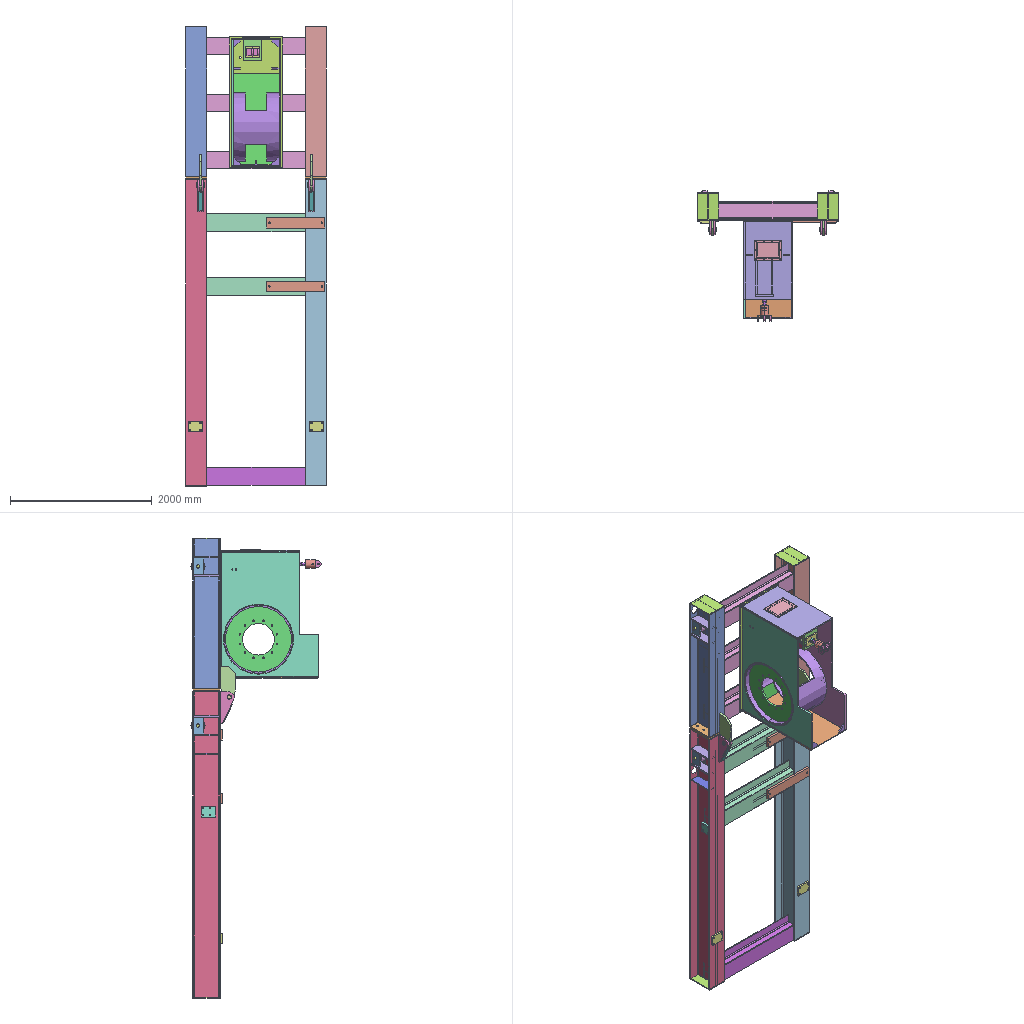Assembly | SolidWorks | 53 different items | 109 placed | box 1991 x 1839 x 6500 mm
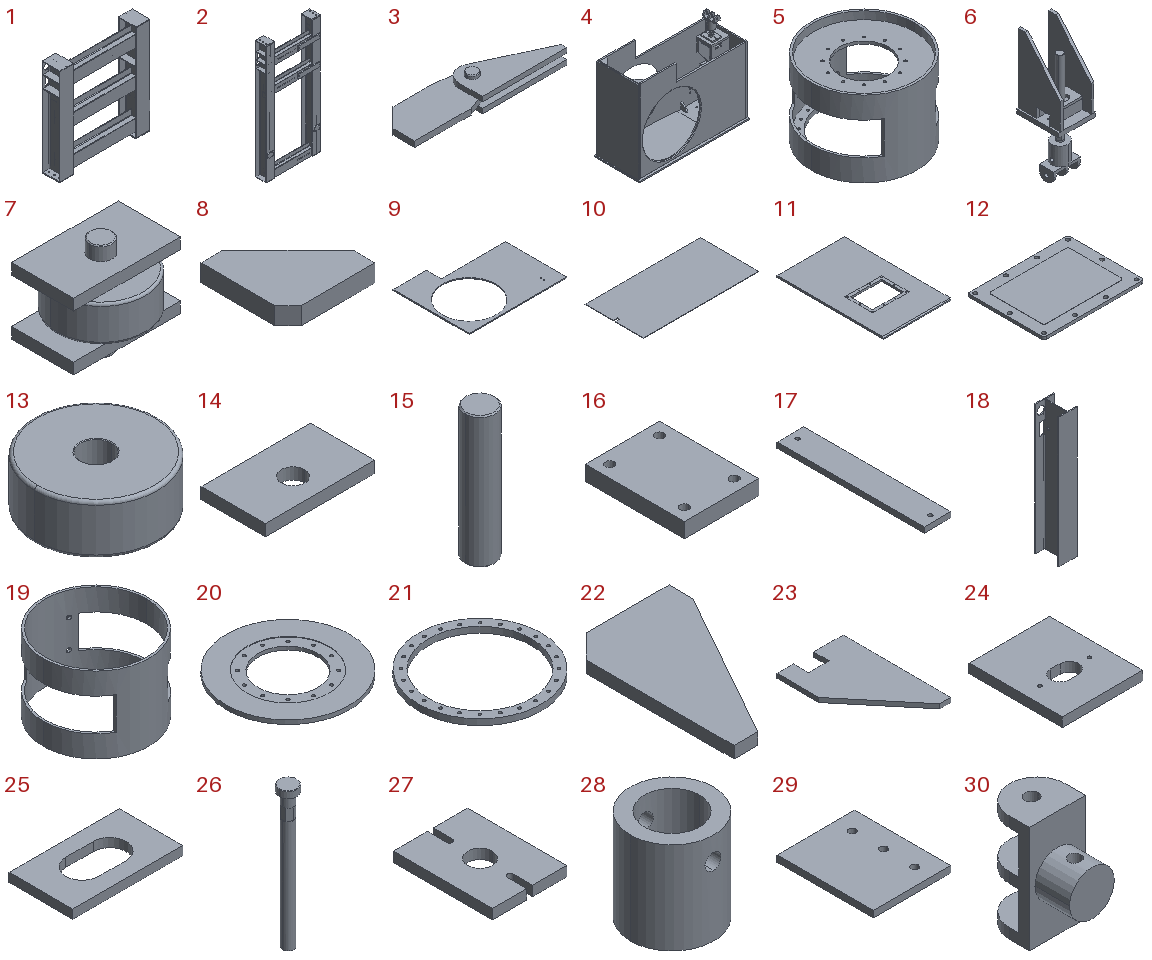Parts list (item | name | quantity | parent item | size | volume | features):
1 | (subassembly) | x1 | - | 1990 x 390 x 2150 mm | 116560797 mm3 | -
2 | (subassembly) | x1 | - | 1990 x 420 x 4350 mm | 182192599 mm3 | -
3 | (subassembly) | x2 | - | 810 x 215 x 108 mm | 5883404 mm3 | features CompositeCurve 1
4 | (subassembly) | x1 | - | 1845 x 760 x 1471 mm | 146946373 mm3 | -
5 | (subassembly) | x1 | - | 970 x 970 x 700 mm | 53801069 mm3 | features ReferencePattern 5, LocalCirPattern 1
6 | (subassembly) | x1 | in 4 | 260 x 300 x 870.542 mm | 11020078 mm3 | -
7 | (subassembly) | x4 | - | 240 x 200 x 220 mm | 4352236 mm3 | -
8 | - | x7 | in 4 | 100 x 100 x 20 mm | 141500 mm3 | features Chamfer 1, Extrusion 1
9 | - | x1 | in 4 | 1775 x 1380 x 25 mm | 34487448 mm3 | features 3DProfileFeature 1, Chamfer 1, Extrusion 1, HoleWzd 1
10 | - | x1 | in 4 | 1286 x 652 x 4 mm | 3349488 mm3 | features Extrusion 1
11 | - | x1 | in 4 | 700 x 1110 x 20 mm | 13982805 mm3 | features 3DProfileFeature 1, Chamfer 1, Extrusion 1, HoleWzd 1, ICE 1
12 | - | x1 | in 4 | 380 x 290 x 12 mm | 1257237 mm3 | features Extrusion 1, ICE 1
13 | - | x4 | in 7 | 200 x 200 x 80 mm | 2343020 mm3 | features Chamfer 1, Extrusion 1, Fillet 1
14 | - | x8 | in 7 | 240 x 140 x 25 mm | 788929 mm3 | features Extrusion 1
15 | - | x4 | in 7 | 50 x 50 x 220 mm | 431357 mm3 | features Chamfer 1, Extrusion 1
16 | - | x2 | in 2 | 150 x 200 x 30 mm | 871137 mm3 | features 3DProfileFeature 1, Extrusion 1, HoleWzd 1
17 | - | x2 | in 2 | 150 x 820 x 30 mm | 3669218 mm3 | features 3DProfileFeature 1, Extrusion 1, HoleWzd 1
18 | - | x1 | in 1 | 300 x 390 x 2113 mm | 27642804 mm3 | features ICE 2, Extrusion 1
19 | - | x1 | in 5 | 970 x 970 x 700 mm | 29802772 mm3 | features ICE 2, Extrusion 1
20 | - | x1 | in 5 | 930 x 930 x 30 mm | 14798488 mm3 | features ICE 2, Extrusion 1
21 | - | x1 | in 5 | 930 x 930 x 45 mm | 8691389 mm3 | features 3DProfileFeature 1, CirPattern 1, Extrusion 1, HoleWzd 1
22 | - | x6 | in 5 | 90 x 145 x 10 mm | 84750 mm3 | features Extrusion 1
23 | - | x2 | in 6 | 300 x 490 x 20 mm | 2058400 mm3 | features Extrusion 1
24 | - | x1 | in 6 | 260 x 300 x 30 mm | 2196274 mm3 | features 3DProfileFeature 1, Extrusion 1, HoleWzd 1
25 | - | x1 | in 6 | 200 x 116 x 16 mm | 277961 mm3 | features Extrusion 1
26 | - | x1 | in 6 | 76 x 76 x 600 mm | 1150657 mm3 | features ICE 3, Chamfer 1, Extrusion 1
27 | - | x1 | in 6 | 150 x 200 x 20 mm | 539748 mm3 | features Extrusion 1
28 | - | x1 | in 6 | 116 x 116 x 128 mm | 818395 mm3 | features ICE 4, Extrusion 1
29 | - | x4 | in 1, 2 | 300 x 370 x 25 mm | 2730453 mm3 | features Extrusion 1
30 | - | x1 | in 6 | 100 x 148 x 191.5 mm | 932566 mm3 | features ICE 3, Extrusion 1
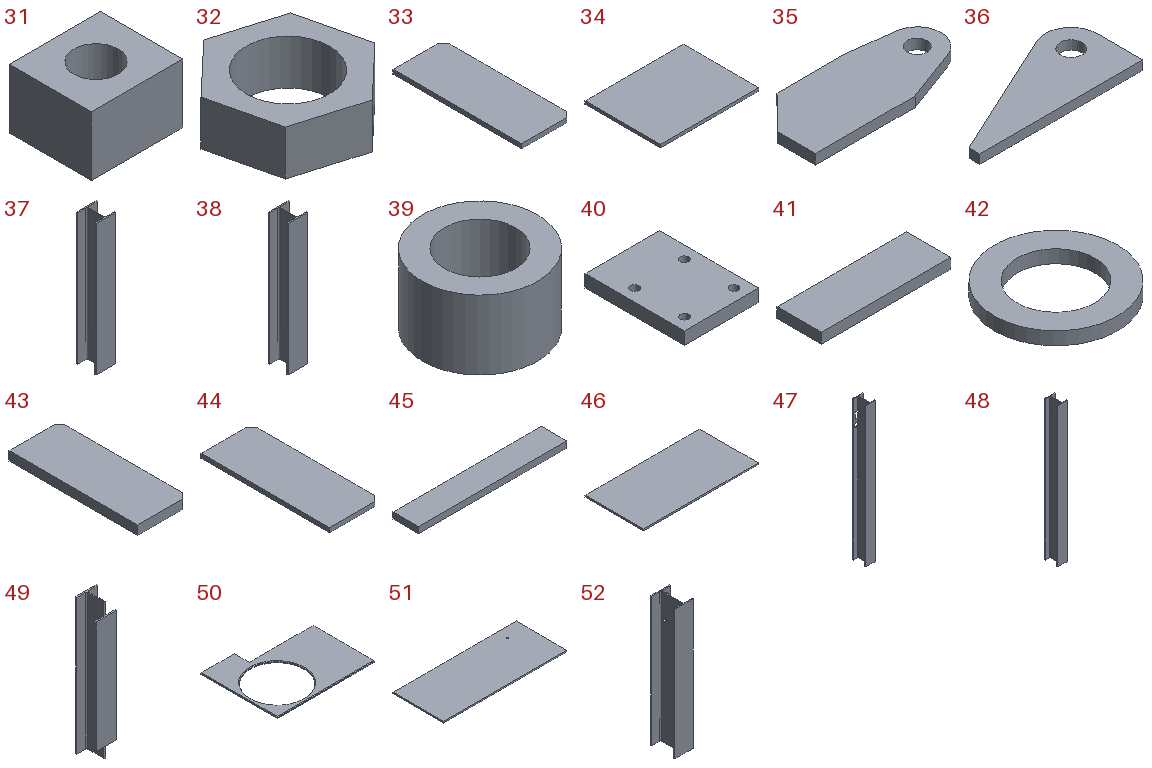31 | - | x1 | in 6 | 100 x 90 x 65 mm | 467379 mm3 | features Extrusion 1
32 | - | x1 | in 6 | 77.461 x 78.628 x 26 mm | 63283 mm3 | features Extrusion 1
33 | - | x2 | in 2 | 140 x 358 x 12 mm | 598740 mm3 | features Chamfer 1, Extrusion 1
34 | - | x4 | in 1, 2 | 390 x 300 x 12 mm | 1404000 mm3 | features Extrusion 1
35 | - | x2 | in 3 | 504 x 215 x 30 mm | 2667245 mm3 | features Extrusion 1
36 | - | x4 | in 3 | 450 x 198 x 25 mm | 1368117 mm3 | features Extrusion 1
37 | - | x1 | in 2 | 250 x 250 x 1681 mm | 15369502 mm3 | features Extrusion 1
38 | - | x3 | in 1 | 250 x 250 x 1681 mm | 15369502 mm3 | features Extrusion 1
39 | - | x1 | in 4 | 50 x 50 x 30 mm | 36626 mm3 | features 3DProfileFeature 1, Extrusion 1, HoleWzd 1
40 | - | x2 | in 1, 2 | 150 x 200 x 25 mm | 728181 mm3 | features 3DProfileFeature 1, Extrusion 1, HoleWzd 1
41 | - | x2 | in 6 | 200 x 68 x 16 mm | 217600 mm3 | features Extrusion 1
42 | - | x1 | in 6 | 76 x 76 x 8 mm | 21815 mm3 | features Extrusion 1
43 | - | x8 | in 1, 2 | 140 x 357 x 25 mm | 1243875 mm3 | features Chamfer 1, Extrusion 1
44 | - | x2 | in 1 | 140 x 357 x 12 mm | 597060 mm3 | features Chamfer 1, Extrusion 1
45 | - | x2 | in 3 | 290 x 50 x 12 mm | 174000 mm3 | features Extrusion 1
46 | - | x1 | in 4 | 1380 x 700 x 20 mm | 19285000 mm3 | features Chamfer 1, Extrusion 1
47 | - | x1 | in 2 | 300 x 390 x 4313 mm | 56956384 mm3 | features ICE 2, Extrusion 1
48 | - | x1 | in 2 | 300 x 390 x 4313 mm | 56957951 mm3 | features ICE 2, Extrusion 1
49 | - | x2 | in 2 | 250 x 250 x 1681 mm | 14328994 mm3 | features Extrusion 1, ICE 1
50 | - | x1 | in 4 | 1775 x 1380 x 25 mm | 34499474 mm3 | features Chamfer 1, Extrusion 1
51 | - | x1 | in 4 | 1845 x 760 x 20 mm | 28037717 mm3 | features Extrusion 1
52 | - | x1 | in 1 | 300 x 390 x 2113 mm | 27642798 mm3 | features ICE 2, Extrusion 1
53 | clevis pins with head gb | x1 | - | - | - | -
Mates (type | each side: item.copy, entity, surface, feature):
In the top assembly
Coincident | 18.1 face plane Boss-Extrude1 | 47.1 face plane Boss-Extrude1
Coincident | 29.1 face plane Boss-Extrude1 | 29.2 face plane Boss-Extrude1
Coincident | 29.3 face plane Boss-Extrude1 | 29.4 face plane Boss-Extrude1
Concentric | 19.1 face cylinder Boss-Extrude1 | 50.1 face cylinder Boss-Extrude1
DistanceDim | 50.1 face cylinder Boss-Extrude1 | 34.1 face plane Boss-Extrude1
Coincident | 19.1 face plane Boss-Extrude1 | 50.1 face plane Boss-Extrude1
Coincident | 48.1 face plane Boss-Extrude1 | 35.1 face plane Boss-Extrude1
Coincident | 47.1 face plane Boss-Extrude1 | 35.2 face plane Boss-Extrude1
Coincident | 48.1 face plane Boss-Extrude1 | 36.1 edge
Coincident | 35.2 face plane Boss-Extrude1 | 35.1 face plane Boss-Extrude1
DistanceDim | 35.1 face plane Boss-Extrude1 | 35.2 face plane Boss-Extrude1
DistanceDim | 35.2 face plane Boss-Extrude1 | 18.1 face plane Boss-Extrude1
Coincident | 38.1 face plane Boss-Extrude1 | 51.1 face plane Boss-Extrude1
Parallel | 52.1 face plane Boss-Extrude1 | 19.1 select_type:24
Coincident | 43.1 face plane Boss-Extrude1 | 14.1 face plane Boss-Extrude1
Concentric | 47.1 face cylinder Cut-Extrude2 | 15.1 face cylinder Boss-Extrude1
Coincident | 47.1 face plane Boss-Extrude1 | 14.2 face plane Boss-Extrude1
Coincident | 43.2 face plane Boss-Extrude1 | 14.3 face plane Boss-Extrude1
Concentric | 48.1 face cylinder Cut-Extrude2 | 15.2 face cylinder Boss-Extrude1
Coincident | 48.1 face plane Boss-Extrude1 | 14.3 face plane Boss-Extrude1
Coincident | 43.3 face plane Boss-Extrude1 | 14.4 face plane Boss-Extrude1
Concentric | 18.1 face cylinder Cut-Extrude2 | 15.3 face cylinder Boss-Extrude1
Coincident | 18.1 face plane Boss-Extrude1 | 14.5 face plane Boss-Extrude1
Coincident | 43.4 face plane Boss-Extrude1 | 14.6 face plane Boss-Extrude1
Coincident | 52.1 face plane Boss-Extrude1 | 14.6 face plane Boss-Extrude1
Concentric | 52.1 face cylinder Cut-Extrude2 | 15.4 face cylinder Boss-Extrude1
In subassembly 2
Coincident | 47.2 face plane Boss-Extrude1 | 48.2 face plane Boss-Extrude1 | 2 times
DistanceDim | 48.2 face plane Boss-Extrude1 | 47.2 face plane Boss-Extrude1
Coincident | 48.2 face plane Boss-Extrude1 | 16.1 face plane Boss-Extrude1
Coincident | 47.2 face plane Boss-Extrude1 | 16.2 face plane Boss-Extrude1
DistanceDim | 16.1 select_type:24 | 48.2 face plane Boss-Extrude1
DistanceDim | 16.2 select_type:24 | 47.2 face plane Boss-Extrude1
Coincident | 16.1 face plane Boss-Extrude1 | 16.2 face plane Boss-Extrude1
Coincident | 47.2 face plane Boss-Extrude1 | 29.5 face plane Boss-Extrude1 | 2 times
DistanceDim | 29.5 face plane Boss-Extrude1 | 47.2 face plane Boss-Extrude1
Coincident | 48.2 face plane Boss-Extrude1 | 29.6 face plane Boss-Extrude1 | 2 times
DistanceDim | 29.6 face plane Boss-Extrude1 | 48.2 face plane Boss-Extrude1
Coincident | 48.2 face plane Boss-Extrude1 | 34.2 face plane Boss-Extrude1 | 3 times
Coincident | 47.2 face plane Boss-Extrude1 | 34.3 face plane Boss-Extrude1 | 3 times
Coincident | 47.2 face plane Boss-Extrude1 | 37.1 face plane Boss-Extrude1 | 2 times
Coincident | 34.3 face plane Boss-Extrude1 | 37.1 face plane Boss-Extrude1
Coincident | 48.2 face plane Boss-Extrude1 | 49.1 face plane Boss-Extrude1 | 2 times
Coincident | 48.2 face plane Boss-Extrude1 | 49.2 face plane Boss-Extrude1 | 2 times
DistanceDim | 49.2 select_type:24 | 29.6 face plane Boss-Extrude1
DistanceDim | 49.2 select_type:24 | 49.1 select_type:24
Coincident | 48.2 face plane Boss-Extrude1 | 17.1 face plane Boss-Extrude1
Coincident | 48.2 face plane Boss-Extrude1 | 17.2 face plane Boss-Extrude1
DistanceDim | 17.1 face plane Boss-Extrude1 | 48.2 face plane Boss-Extrude1
Coincident | 17.2 face plane Boss-Extrude1 | 17.1 face plane Boss-Extrude1
DistanceDim | 17.2 face plane Boss-Extrude1 | 17.1 face plane Boss-Extrude1
DistanceDim | 17.1 face plane Boss-Extrude1 | 49.2 select_type:24
Coincident | 47.2 face plane Boss-Extrude1 | 43.5 face plane Boss-Extrude1 | 2 times
Coincident | 47.2 face plane Boss-Extrude1 | 43.6 face plane Boss-Extrude1
Coincident | 43.5 face plane Boss-Extrude1 | 43.6 face plane Boss-Extrude1
Coincident | 43.6 face plane Boss-Extrude1 | 33.1 face plane Boss-Extrude1
Coincident | 47.2 face plane Boss-Extrude1 | 33.1 face plane Boss-Extrude1
DistanceDim | 43.5 face plane Boss-Extrude1 | 29.5 face plane Boss-Extrude1
DistanceDim | 43.5 face plane Boss-Extrude1 | 43.6 face plane Boss-Extrude1
DistanceDim | 43.6 face plane Boss-Extrude1 | 33.1 face plane Boss-Extrude1
Coincident | 47.2 face plane Boss-Extrude1 | 40.1 face plane Boss-Extrude1
DistanceDim | 40.1 face plane Boss-Extrude1 | 29.5 face plane Boss-Extrude1
DistanceDim | 40.1 face plane Boss-Extrude1 | 47.2 face plane Boss-Extrude1
Coincident | 48.2 face plane Boss-Extrude1 | 33.2 face plane Boss-Extrude1 | 2 times
Coincident | 33.1 face plane Boss-Extrude1 | 33.2 face plane Boss-Extrude1
Coincident | 43.5 face plane Boss-Extrude1 | 43.7 face plane Boss-Extrude1
Coincident | 43.6 face plane Boss-Extrude1 | 43.8 face plane Boss-Extrude1
Coincident | 48.2 face plane Boss-Extrude1 | 43.7 face plane Boss-Extrude1 | 2 times
Coincident | 48.2 face plane Boss-Extrude1 | 43.8 face plane Boss-Extrude1 | 2 times
In subassembly 3
Concentric | 35.3 face cylinder Boss-Extrude1 | 36.2 face cylinder Boss-Extrude1
Concentric | 36.3 face cylinder Boss-Extrude1 | 36.2 face cylinder Boss-Extrude1
Coincident | 35.3 face plane Boss-Extrude1 | 36.3 face plane Boss-Extrude1
Coincident | 35.3 face plane Boss-Extrude1 | 36.2 face plane Boss-Extrude1 | 2 times
Coincident | 36.3 face plane Boss-Extrude1 | 36.2 face plane Boss-Extrude1
Coincident | 36.3 face plane Boss-Extrude1 | 45.1 face plane Boss-Extrude1
DistanceDim | 45.1 face plane Boss-Extrude1 | 36.3 edge
DistanceDim | 45.1 face plane Boss-Extrude1 | 36.2 face plane Boss-Extrude1
In subassembly 1
Coincident | 52.2 face plane Boss-Extrude1 | 18.2 face plane Boss-Extrude1 | 2 times
DistanceDim | 52.2 face plane Boss-Extrude1 | 18.2 face plane Boss-Extrude1
Coincident | 52.2 face plane Boss-Extrude1 | 34.2 face plane Boss-Extrude1 | 3 times
Coincident | 18.2 face plane Boss-Extrude1 | 34.3 face plane Boss-Extrude1 | 3 times
Coincident | 18.2 face plane Boss-Extrude1 | 38.2 face plane Boss-Extrude1
Coincident | 52.2 face plane Boss-Extrude1 | 38.2 face plane Boss-Extrude1
DistanceDim | 38.2 select_type:24 | 34.3 face plane Boss-Extrude1
Coincident | 38.2 face plane Boss-Extrude1 | 38.3 face plane Boss-Extrude1
Coincident | 38.2 face plane Boss-Extrude1 | 38.4 face plane Boss-Extrude1
Coincident | 18.2 face plane Boss-Extrude1 | 38.3 face plane Boss-Extrude1
Coincident | 18.2 face plane Boss-Extrude1 | 38.4 face plane Boss-Extrude1
DistanceDim | 38.3 select_type:24 | 38.2 select_type:24
DistanceDim | 38.4 select_type:24 | 38.3 select_type:24
Coincident | 52.2 face plane Boss-Extrude1 | 40.1 face plane Boss-Extrude1
Coincident | 52.2 face plane Boss-Extrude1 | 29.5 face plane Boss-Extrude1 | 2 times
Coincident | 29.5 face plane Boss-Extrude1 | 29.6 face plane Boss-Extrude1 | 2 times
Coincident | 18.2 face plane Boss-Extrude1 | 29.6 face plane Boss-Extrude1
DistanceDim | 29.6 face plane Boss-Extrude1 | 18.2 face plane Boss-Extrude1
Coincident | 52.2 face plane Boss-Extrude1 | 43.6 face plane Boss-Extrude1 | 2 times
Coincident | 52.2 face plane Boss-Extrude1 | 43.5 face plane Boss-Extrude1
Coincident | 43.5 face plane Boss-Extrude1 | 43.6 face plane Boss-Extrude1
DistanceDim | 43.5 face plane Boss-Extrude1 | 34.2 face plane Boss-Extrude1
DistanceDim | 43.5 face plane Boss-Extrude1 | 43.6 face plane Boss-Extrude1
Coincident | 52.2 face plane Boss-Extrude1 | 44.1 face plane Boss-Extrude1 | 2 times
Coincident | 44.2 face plane Boss-Extrude1 | 44.1 face plane Boss-Extrude1
Coincident | 18.2 face plane Boss-Extrude1 | 44.2 face plane Boss-Extrude1 | 2 times
Coincident | 43.6 face plane Boss-Extrude1 | 43.8 face plane Boss-Extrude1
Coincident | 18.2 face plane Boss-Extrude1 | 43.8 face plane Boss-Extrude1 | 2 times
Coincident | 43.7 face plane Boss-Extrude1 | 43.8 face plane Boss-Extrude1
Coincident | 43.5 face plane Boss-Extrude1 | 43.7 face plane Boss-Extrude1
Coincident | 18.2 face plane Boss-Extrude1 | 43.7 face plane Boss-Extrude1
DistanceDim | 44.2 face plane Boss-Extrude1 | 34.3 face plane Boss-Extrude1
In subassembly 4
Coincident | 51.2 face plane Boss-Extrude1 | 50.2 face plane Boss-Extrude1
Coincident | 51.2 face plane Boss-Extrude1 | 9.1 face plane Boss-Extrude1
Coincident | 50.2 face plane Boss-Extrude1 | 9.1 face plane Boss-Extrude1
DistanceDim | 50.2 face plane Boss-Extrude1 | 9.1 face plane Boss-Extrude1
DistanceDim | 50.2 face plane Boss-Extrude1 | 51.2 face plane Boss-Extrude1
Coincident | 51.2 face plane Boss-Extrude1 | 46.1 face plane Boss-Extrude1
Coincident | 50.2 face plane Boss-Extrude1 | 46.1 face plane Boss-Extrude1 | 2 times
DistanceDim | 46.1 face plane Boss-Extrude1 | 51.2 face plane Boss-Extrude1
Coincident | 51.2 face plane Boss-Extrude1 | 11.1 face plane Boss-Extrude1
Coincident | 50.2 face plane Boss-Extrude1 | 11.1 face plane Boss-Extrude1 | 2 times
Coincident | 11.1 face plane Boss-Extrude1 | 24.1 face plane Boss-Extrude1
DistanceDim | 24.1 face plane Boss-Extrude1 | 11.1 face plane Boss-Extrude1
DistanceDim | 28.1 face cylinder Cut-Extrude1 | 9.1 face plane Boss-Extrude1
Coincident | 51.2 face plane Boss-Extrude1 | 39.1 face plane Boss-Extrude1
Concentric | 51.2 face cylinder Boss-Extrude1 | 39.1 face cylinder G1 Threaded hole1
Coincident | 50.2 face plane Boss-Extrude1 | 8.1 face plane Boss-Extrude1
Coincident | 11.1 face plane Boss-Extrude1 | 8.1 face plane Boss-Extrude1
DistanceDim | 8.1 face plane Boss-Extrude1 | 51.2 face plane Boss-Extrude1
Coincident | 9.1 face plane Boss-Extrude1 | 8.2 face plane Boss-Extrude1
Coincident | 11.1 face plane Boss-Extrude1 | 8.2 face plane Boss-Extrude1
Coincident | 8.1 face plane Boss-Extrude1 | 8.2 face plane Boss-Extrude1
Coincident | 50.2 face plane Boss-Extrude1 | 8.3 face plane Boss-Extrude1 | 2 times
Coincident | 46.1 face plane Boss-Extrude1 | 8.3 face plane Boss-Extrude1
Coincident | 46.1 face plane Boss-Extrude1 | 8.4 face plane Boss-Extrude1
Coincident | 8.3 face plane Boss-Extrude1 | 8.4 face plane Boss-Extrude1
Coincident | 9.1 face plane Boss-Extrude1 | 8.4 face plane Boss-Extrude1
Coincident | 51.2 face plane Boss-Extrude1 | 8.5 face plane Boss-Extrude1
Coincident | 50.2 face plane Boss-Extrude1 | 8.5 face plane Boss-Extrude1
Coincident | 51.2 face plane Boss-Extrude1 | 8.6 face plane Boss-Extrude1
Coincident | 9.1 face plane Boss-Extrude1 | 8.6 face plane Boss-Extrude1
DistanceDim | 8.6 face plane Boss-Extrude1 | 11.1 face plane Boss-Extrude1
Coincident | 8.5 face plane Boss-Extrude1 | 8.6 face plane Boss-Extrude1
Coincident | 51.2 face plane Boss-Extrude1 | 8.7 face plane Boss-Extrude1
Coincident | 46.1 face plane Boss-Extrude1 | 8.7 face plane Boss-Extrude1
Coincident | 51.2 face plane Boss-Extrude1 | 10.1 edge
Coincident | 9.1 face plane Boss-Extrude1 | 10.1 face plane Boss-Extrude1
DistanceDim | 10.1 edge | 8.6 face plane Boss-Extrude1
DistanceDim | 10.1 edge | 51.2 face plane Boss-Extrude1
Coincident | 11.1 face plane Cut-Extrude1 | 12.1 face plane Cut-Extrude1
Concentric | 11.1 face cylinder 1/2-13 Threaded hole1 | 12.1 face cylinder Boss-Extrude1 | 2 times
In subassembly 6
Coincident | 24.2 face plane Boss-Extrude1 | 23.1 face plane Boss-Extrude1 | 2 times
Coincident | 24.2 face plane Boss-Extrude1 | 23.2 face plane Boss-Extrude1
Coincident | 23.2 face plane Boss-Extrude1 | 23.1 face plane Boss-Extrude1
Coincident | 24.2 face plane Boss-Extrude1 | 41.1 face plane Boss-Extrude1
Coincident | 41.1 face plane Boss-Extrude1 | 41.2 face plane Boss-Extrude1 | 2 times
DistanceDim | 23.1 face plane Boss-Extrude1 | 24.2 face plane Boss-Extrude1
DistanceDim | 23.2 face plane Boss-Extrude1 | 24.2 face plane Boss-Extrude1
Coincident | 23.2 face plane Boss-Extrude1 | 41.1 face plane Boss-Extrude1
Coincident | 24.2 face plane Boss-Extrude1 | 27.1 face plane Boss-Extrude1
DistanceDim | 27.1 face plane Boss-Extrude1 | 24.2 face plane Boss-Extrude1 | 2 times
Concentric | 27.1 face cylinder Boss-Extrude1 | 26.1 face cylinder Boss-Extrude3
Coincident | 24.2 face plane Boss-Extrude1 | 31.1 face plane Boss-Extrude1
Concentric | 26.1 face cylinder Boss-Extrude4 | 31.1 face cylinder Boss-Extrude1
Coincident | 41.2 face plane Boss-Extrude1 | 31.1 face plane Boss-Extrude1
Coincident | 41.1 face plane Boss-Extrude1 | 31.1 face plane Boss-Extrude1
Concentric | 26.1 face cylinder Boss-Extrude3 | 28.2 face cylinder Boss-Extrude1
Concentric | 26.1 face cylinder Boss-Extrude2 | 42.1 face cylinder Boss-Extrude1
Coincident | 26.1 face plane Boss-Extrude3 | 42.1 face plane Boss-Extrude1
Coincident | 28.2 face plane Cut-Extrude1 | 42.1 face plane Boss-Extrude1
Coincident | 23.2 face plane Boss-Extrude1 | 25.1 face plane Boss-Extrude1
Coincident | 41.1 face plane Boss-Extrude1 | 25.1 face plane Boss-Extrude1
Concentric | 28.2 face cylinder Cut-Extrude3 | 30.1 face cylinder Boss-Extrude2
Concentric | 28.2 face cylinder Cut-Extrude2 | 30.1 face cylinder Cut-Extrude8
Concentric | 26.1 face cylinder Boss-Extrude4 | 32.1 face cylinder Boss-Extrude1
Coincident | 27.1 face plane Boss-Extrude1 | 32.1 face plane Boss-Extrude1
Parallel | 23.2 face plane Boss-Extrude1 | 30.1 face plane Boss-Extrude1
In subassembly 7
Concentric | 14.7 face cylinder Boss-Extrude1 | 14.8 face cylinder Boss-Extrude1
Coincident | 14.7 face plane Boss-Extrude1 | 14.8 face plane Boss-Extrude1
Concentric | 14.8 face cylinder Boss-Extrude1 | 15.5 face cylinder Boss-Extrude1
Concentric | 15.5 face cylinder Boss-Extrude1 | 13.1 face cylinder Boss-Extrude1
DistanceDim | 13.1 face plane Boss-Extrude1 | 14.8 face plane Boss-Extrude1
DistanceDim | 14.7 face plane Boss-Extrude1 | 13.1 face plane Boss-Extrude1
In subassembly 5
DistanceDim | 19.2 select_type:24 | 21.1 face plane Boss-Extrude1
Concentric | 19.2 face cylinder Boss-Extrude1 | 21.1 face cylinder Boss-Extrude1
DistanceDim | 20.1 face plane Cut-Extrude1 | 21.1 face plane Boss-Extrude1
Concentric | 19.2 face cylinder Boss-Extrude1 | 20.1 face cylinder Boss-Extrude1
Parallel | 19.2 select_type:24 | 20.1 select_type:24
Parallel | 19.2 select_type:24 | 21.1 select_type:24
Coincident | 20.1 face plane Boss-Extrude1 | 22.1 face plane Boss-Extrude1
Coincident | 20.1 select_type:24 | 22.1 select_type:24
Coincident | 19.2 face cylinder Boss-Extrude1 | 22.1 edge